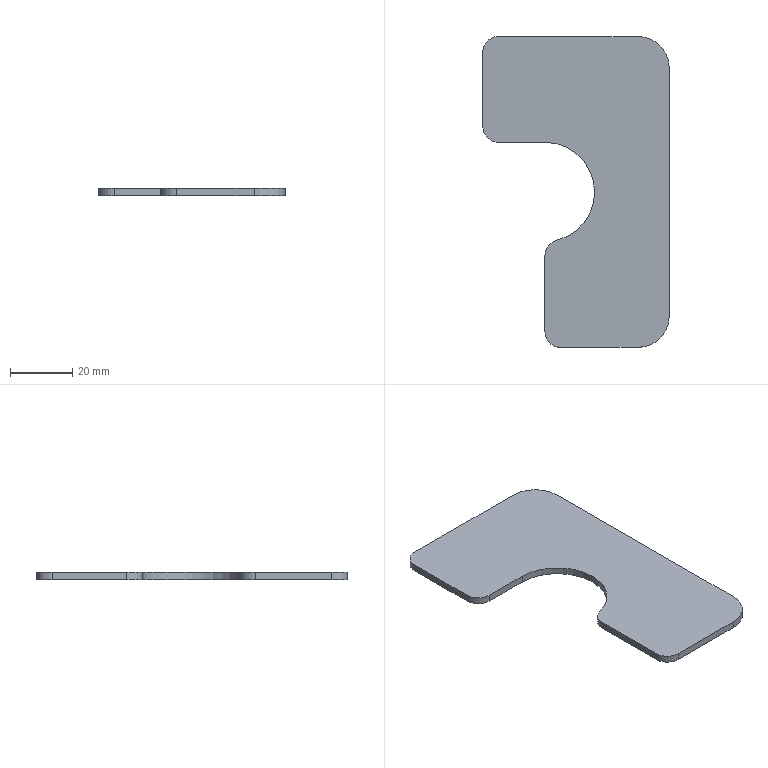Part | SolidWorks | features FlatPattern 1, SMBaseFlange 1, SheetMetal 1 | 1 solid | 15 faces | box 60 x 100 x 2.3 mm | volume 9695 mm3 | plane 8 | cylinder 7 | commonest cylinder face diameters 10 x4 20 x2 32 x1
STEP:
#1=CARTESIAN_POINT('',(247.5,0.,0.));
#2=VERTEX_POINT('',#1);
#3=CARTESIAN_POINT('',(252.5,-5.,0.));
#4=VERTEX_POINT('',#3);
#5=CARTESIAN_POINT('',(252.5,0.,0.));
#6=DIRECTION('',(0.,0.,1.));
#7=DIRECTION('',(1.,0.,0.));
#8=AXIS2_PLACEMENT_3D('',#5,#6,#7);
#9=CIRCLE('',#8,5.);
#10=EDGE_CURVE('',#2,#4,#9,.T.);
#11=ORIENTED_EDGE('',*,*,#10,.T.);
#12=CARTESIAN_POINT('',(252.5,-5.,2.3));
#13=VERTEX_POINT('',#12);
#14=CARTESIAN_POINT('',(252.5,-5.,2.3));
#15=DIRECTION('',(0.,0.,-1.));
#16=VECTOR('',#15,1000.);
#17=LINE('',#14,#16);
#18=EDGE_CURVE('',#13,#4,#17,.T.);
#19=ORIENTED_EDGE('',*,*,#18,.F.);
#20=CARTESIAN_POINT('',(247.5,0.,2.3));
#21=VERTEX_POINT('',#20);
#22=CARTESIAN_POINT('',(252.5,0.,2.3));
#23=DIRECTION('',(0.,0.,1.));
#24=DIRECTION('',(1.,0.,0.));
#25=AXIS2_PLACEMENT_3D('',#22,#23,#24);
#26=CIRCLE('',#25,5.);
#27=EDGE_CURVE('',#21,#13,#26,.T.);
#28=ORIENTED_EDGE('',*,*,#27,.F.);
#29=CARTESIAN_POINT('',(247.5,0.,2.3));
#30=DIRECTION('',(0.,0.,-1.));
#31=VECTOR('',#30,1000.);
#32=LINE('',#29,#31);
#33=EDGE_CURVE('',#21,#2,#32,.T.);
#34=ORIENTED_EDGE('',*,*,#33,.T.);
#35=EDGE_LOOP('',(#11,#19,#28,#34));
#36=FACE_OUTER_BOUND('',#35,.T.);
#37=CARTESIAN_POINT('',(252.5,0.,2.3));
#38=DIRECTION('',(0.,0.,-1.));
#39=DIRECTION('',(-1.,0.,0.));
#40=AXIS2_PLACEMENT_3D('',#37,#38,#39);
#41=CYLINDRICAL_SURFACE('',#40,5.);
#42=ADVANCED_FACE('',(#36),#41,.T.);
#43=CARTESIAN_POINT('',(277.5,-5.,0.));
#44=VERTEX_POINT('',#43);
#45=CARTESIAN_POINT('',(252.5,-5.,0.));
#46=DIRECTION('',(1.,0.,0.));
#47=VECTOR('',#46,1000.);
#48=LINE('',#45,#47);
#49=EDGE_CURVE('',#4,#44,#48,.T.);
#50=ORIENTED_EDGE('',*,*,#49,.T.);
#51=CARTESIAN_POINT('',(277.5,-5.,2.3));
#52=VERTEX_POINT('',#51);
#53=CARTESIAN_POINT('',(277.5,-5.,2.3));
#54=DIRECTION('',(0.,0.,-1.));
#55=VECTOR('',#54,1000.);
#56=LINE('',#53,#55);
#57=EDGE_CURVE('',#52,#44,#56,.T.);
#58=ORIENTED_EDGE('',*,*,#57,.F.);
#59=CARTESIAN_POINT('',(252.5,-5.,2.3));
#60=DIRECTION('',(1.,0.,0.));
#61=VECTOR('',#60,1000.);
#62=LINE('',#59,#61);
#63=EDGE_CURVE('',#13,#52,#62,.T.);
#64=ORIENTED_EDGE('',*,*,#63,.F.);
#65=ORIENTED_EDGE('',*,*,#18,.T.);
#66=EDGE_LOOP('',(#50,#58,#64,#65));
#67=FACE_OUTER_BOUND('',#66,.T.);
#68=CARTESIAN_POINT('',(252.5,-5.,2.3));
#69=DIRECTION('',(0.,1.,0.));
#70=DIRECTION('',(0.,0.,1.));
#71=AXIS2_PLACEMENT_3D('',#68,#69,#70);
#72=PLANE('',#71);
#73=ADVANCED_FACE('',(#67),#72,.F.);
#74=CARTESIAN_POINT('',(287.5,5.,0.));
#75=VERTEX_POINT('',#74);
#76=CARTESIAN_POINT('',(277.5,5.,0.));
#77=DIRECTION('',(0.,0.,1.));
#78=DIRECTION('',(-1.,0.,0.));
#79=AXIS2_PLACEMENT_3D('',#76,#77,#78);
#80=CIRCLE('',#79,10.);
#81=EDGE_CURVE('',#44,#75,#80,.T.);
#82=ORIENTED_EDGE('',*,*,#81,.T.);
#83=CARTESIAN_POINT('',(287.5,5.,2.3));
#84=VERTEX_POINT('',#83);
#85=CARTESIAN_POINT('',(287.5,5.,2.3));
#86=DIRECTION('',(0.,0.,-1.));
#87=VECTOR('',#86,1000.);
#88=LINE('',#85,#87);
#89=EDGE_CURVE('',#84,#75,#88,.T.);
#90=ORIENTED_EDGE('',*,*,#89,.F.);
#91=CARTESIAN_POINT('',(277.5,5.,2.3));
#92=DIRECTION('',(0.,0.,1.));
#93=DIRECTION('',(-1.,0.,0.));
#94=AXIS2_PLACEMENT_3D('',#91,#92,#93);
#95=CIRCLE('',#94,10.);
#96=EDGE_CURVE('',#52,#84,#95,.T.);
#97=ORIENTED_EDGE('',*,*,#96,.F.);
#98=ORIENTED_EDGE('',*,*,#57,.T.);
#99=EDGE_LOOP('',(#82,#90,#97,#98));
#100=FACE_OUTER_BOUND('',#99,.T.);
#101=CARTESIAN_POINT('',(277.5,5.,2.3));
#102=DIRECTION('',(0.,0.,-1.));
#103=DIRECTION('',(-1.,0.,0.));
#104=AXIS2_PLACEMENT_3D('',#101,#102,#103);
#105=CYLINDRICAL_SURFACE('',#104,10.);
#106=ADVANCED_FACE('',(#100),#105,.T.);
#107=CARTESIAN_POINT('',(287.5,85.,0.));
#108=VERTEX_POINT('',#107);
#109=CARTESIAN_POINT('',(287.5,85.,0.));
#110=DIRECTION('',(0.,1.,0.));
#111=VECTOR('',#110,1000.);
#112=LINE('',#109,#111);
#113=EDGE_CURVE('',#75,#108,#112,.T.);
#114=ORIENTED_EDGE('',*,*,#113,.T.);
#115=CARTESIAN_POINT('',(287.5,85.,2.3));
#116=VERTEX_POINT('',#115);
#117=CARTESIAN_POINT('',(287.5,85.,2.3));
#118=DIRECTION('',(0.,0.,-1.));
#119=VECTOR('',#118,1000.);
#120=LINE('',#117,#119);
#121=EDGE_CURVE('',#116,#108,#120,.T.);
#122=ORIENTED_EDGE('',*,*,#121,.F.);
#123=CARTESIAN_POINT('',(287.5,85.,2.3));
#124=DIRECTION('',(0.,1.,0.));
#125=VECTOR('',#124,1000.);
#126=LINE('',#123,#125);
#127=EDGE_CURVE('',#84,#116,#126,.T.);
#128=ORIENTED_EDGE('',*,*,#127,.F.);
#129=ORIENTED_EDGE('',*,*,#89,.T.);
#130=EDGE_LOOP('',(#114,#122,#128,#129));
#131=FACE_OUTER_BOUND('',#130,.T.);
#132=CARTESIAN_POINT('',(287.5,85.,2.3));
#133=DIRECTION('',(-1.,0.,0.));
#134=DIRECTION('',(0.,0.,1.));
#135=AXIS2_PLACEMENT_3D('',#132,#133,#134);
#136=PLANE('',#135);
#137=ADVANCED_FACE('',(#131),#136,.F.);
#138=CARTESIAN_POINT('',(277.5,95.,0.));
#139=VERTEX_POINT('',#138);
#140=CARTESIAN_POINT('',(277.5,85.,0.));
#141=DIRECTION('',(0.,0.,1.));
#142=DIRECTION('',(-1.,0.,0.));
#143=AXIS2_PLACEMENT_3D('',#140,#141,#142);
#144=CIRCLE('',#143,10.);
#145=EDGE_CURVE('',#108,#139,#144,.T.);
#146=ORIENTED_EDGE('',*,*,#145,.T.);
#147=CARTESIAN_POINT('',(277.5,95.,2.3));
#148=VERTEX_POINT('',#147);
#149=CARTESIAN_POINT('',(277.5,95.,2.3));
#150=DIRECTION('',(0.,0.,-1.));
#151=VECTOR('',#150,1000.);
#152=LINE('',#149,#151);
#153=EDGE_CURVE('',#148,#139,#152,.T.);
#154=ORIENTED_EDGE('',*,*,#153,.F.);
#155=CARTESIAN_POINT('',(277.5,85.,2.3));
#156=DIRECTION('',(0.,0.,1.));
#157=DIRECTION('',(-1.,0.,0.));
#158=AXIS2_PLACEMENT_3D('',#155,#156,#157);
#159=CIRCLE('',#158,10.);
#160=EDGE_CURVE('',#116,#148,#159,.T.);
#161=ORIENTED_EDGE('',*,*,#160,.F.);
#162=ORIENTED_EDGE('',*,*,#121,.T.);
#163=EDGE_LOOP('',(#146,#154,#161,#162));
#164=FACE_OUTER_BOUND('',#163,.T.);
#165=CARTESIAN_POINT('',(277.5,85.,2.3));
#166=DIRECTION('',(0.,0.,-1.));
#167=DIRECTION('',(-1.,0.,0.));
#168=AXIS2_PLACEMENT_3D('',#165,#166,#167);
#169=CYLINDRICAL_SURFACE('',#168,10.);
#170=ADVANCED_FACE('',(#164),#169,.T.);
#171=CARTESIAN_POINT('',(232.5,95.,0.));
#172=VERTEX_POINT('',#171);
#173=CARTESIAN_POINT('',(277.5,95.,0.));
#174=DIRECTION('',(-1.,0.,0.));
#175=VECTOR('',#174,1000.);
#176=LINE('',#173,#175);
#177=EDGE_CURVE('',#139,#172,#176,.T.);
#178=ORIENTED_EDGE('',*,*,#177,.T.);
#179=CARTESIAN_POINT('',(232.5,95.,2.3));
#180=VERTEX_POINT('',#179);
#181=CARTESIAN_POINT('',(232.5,95.,2.3));
#182=DIRECTION('',(0.,0.,-1.));
#183=VECTOR('',#182,1000.);
#184=LINE('',#181,#183);
#185=EDGE_CURVE('',#180,#172,#184,.T.);
#186=ORIENTED_EDGE('',*,*,#185,.F.);
#187=CARTESIAN_POINT('',(277.5,95.,2.3));
#188=DIRECTION('',(-1.,0.,0.));
#189=VECTOR('',#188,1000.);
#190=LINE('',#187,#189);
#191=EDGE_CURVE('',#148,#180,#190,.T.);
#192=ORIENTED_EDGE('',*,*,#191,.F.);
#193=ORIENTED_EDGE('',*,*,#153,.T.);
#194=EDGE_LOOP('',(#178,#186,#192,#193));
#195=FACE_OUTER_BOUND('',#194,.T.);
#196=CARTESIAN_POINT('',(277.5,95.,2.3));
#197=DIRECTION('',(0.,-1.,0.));
#198=DIRECTION('',(0.,0.,-1.));
#199=AXIS2_PLACEMENT_3D('',#196,#197,#198);
#200=PLANE('',#199);
#201=ADVANCED_FACE('',(#195),#200,.F.);
#202=CARTESIAN_POINT('',(227.5,90.,0.));
#203=VERTEX_POINT('',#202);
#204=CARTESIAN_POINT('',(232.5,90.,0.));
#205=DIRECTION('',(0.,0.,1.));
#206=DIRECTION('',(1.,0.,0.));
#207=AXIS2_PLACEMENT_3D('',#204,#205,#206);
#208=CIRCLE('',#207,5.);
#209=EDGE_CURVE('',#172,#203,#208,.T.);
#210=ORIENTED_EDGE('',*,*,#209,.T.);
#211=CARTESIAN_POINT('',(227.5,90.,2.3));
#212=VERTEX_POINT('',#211);
#213=CARTESIAN_POINT('',(227.5,90.,2.3));
#214=DIRECTION('',(0.,0.,-1.));
#215=VECTOR('',#214,1000.);
#216=LINE('',#213,#215);
#217=EDGE_CURVE('',#212,#203,#216,.T.);
#218=ORIENTED_EDGE('',*,*,#217,.F.);
#219=CARTESIAN_POINT('',(232.5,90.,2.3));
#220=DIRECTION('',(0.,0.,1.));
#221=DIRECTION('',(1.,0.,0.));
#222=AXIS2_PLACEMENT_3D('',#219,#220,#221);
#223=CIRCLE('',#222,5.);
#224=EDGE_CURVE('',#180,#212,#223,.T.);
#225=ORIENTED_EDGE('',*,*,#224,.F.);
#226=ORIENTED_EDGE('',*,*,#185,.T.);
#227=EDGE_LOOP('',(#210,#218,#225,#226));
#228=FACE_OUTER_BOUND('',#227,.T.);
#229=CARTESIAN_POINT('',(232.5,90.,2.3));
#230=DIRECTION('',(0.,0.,-1.));
#231=DIRECTION('',(-1.,0.,0.));
#232=AXIS2_PLACEMENT_3D('',#229,#230,#231);
#233=CYLINDRICAL_SURFACE('',#232,5.);
#234=ADVANCED_FACE('',(#228),#233,.T.);
#235=CARTESIAN_POINT('',(227.5,66.,0.));
#236=VERTEX_POINT('',#235);
#237=CARTESIAN_POINT('',(227.5,90.,0.));
#238=DIRECTION('',(0.,-1.,0.));
#239=VECTOR('',#238,1000.);
#240=LINE('',#237,#239);
#241=EDGE_CURVE('',#203,#236,#240,.T.);
#242=ORIENTED_EDGE('',*,*,#241,.T.);
#243=CARTESIAN_POINT('',(227.5,66.,2.3));
#244=VERTEX_POINT('',#243);
#245=CARTESIAN_POINT('',(227.5,66.,2.3));
#246=DIRECTION('',(0.,0.,-1.));
#247=VECTOR('',#246,1000.);
#248=LINE('',#245,#247);
#249=EDGE_CURVE('',#244,#236,#248,.T.);
#250=ORIENTED_EDGE('',*,*,#249,.F.);
#251=CARTESIAN_POINT('',(227.5,90.,2.3));
#252=DIRECTION('',(0.,-1.,0.));
#253=VECTOR('',#252,1000.);
#254=LINE('',#251,#253);
#255=EDGE_CURVE('',#212,#244,#254,.T.);
#256=ORIENTED_EDGE('',*,*,#255,.F.);
#257=ORIENTED_EDGE('',*,*,#217,.T.);
#258=EDGE_LOOP('',(#242,#250,#256,#257));
#259=FACE_OUTER_BOUND('',#258,.T.);
#260=CARTESIAN_POINT('',(227.5,90.,2.3));
#261=DIRECTION('',(1.,0.,0.));
#262=DIRECTION('',(0.,0.,-1.));
#263=AXIS2_PLACEMENT_3D('',#260,#261,#262);
#264=PLANE('',#263);
#265=ADVANCED_FACE('',(#259),#264,.F.);
#266=CARTESIAN_POINT('',(232.5,61.,0.));
#267=VERTEX_POINT('',#266);
#268=CARTESIAN_POINT('',(232.5,66.,0.));
#269=DIRECTION('',(0.,0.,1.));
#270=DIRECTION('',(1.,0.,0.));
#271=AXIS2_PLACEMENT_3D('',#268,#269,#270);
#272=CIRCLE('',#271,5.);
#273=EDGE_CURVE('',#236,#267,#272,.T.);
#274=ORIENTED_EDGE('',*,*,#273,.T.);
#275=CARTESIAN_POINT('',(232.5,61.,2.3));
#276=VERTEX_POINT('',#275);
#277=CARTESIAN_POINT('',(232.5,61.,2.3));
#278=DIRECTION('',(0.,0.,-1.));
#279=VECTOR('',#278,1000.);
#280=LINE('',#277,#279);
#281=EDGE_CURVE('',#276,#267,#280,.T.);
#282=ORIENTED_EDGE('',*,*,#281,.F.);
#283=CARTESIAN_POINT('',(232.5,66.,2.3));
#284=DIRECTION('',(0.,0.,1.));
#285=DIRECTION('',(1.,0.,0.));
#286=AXIS2_PLACEMENT_3D('',#283,#284,#285);
#287=CIRCLE('',#286,5.);
#288=EDGE_CURVE('',#244,#276,#287,.T.);
#289=ORIENTED_EDGE('',*,*,#288,.F.);
#290=ORIENTED_EDGE('',*,*,#249,.T.);
#291=EDGE_LOOP('',(#274,#282,#289,#290));
#292=FACE_OUTER_BOUND('',#291,.T.);
#293=CARTESIAN_POINT('',(232.5,66.,2.3));
#294=DIRECTION('',(0.,0.,-1.));
#295=DIRECTION('',(-1.,0.,0.));
#296=AXIS2_PLACEMENT_3D('',#293,#294,#295);
#297=CYLINDRICAL_SURFACE('',#296,5.);
#298=ADVANCED_FACE('',(#292),#297,.T.);
#299=CARTESIAN_POINT('',(247.5,61.,0.));
#300=VERTEX_POINT('',#299);
#301=CARTESIAN_POINT('',(232.5,61.,0.));
#302=DIRECTION('',(1.,0.,0.));
#303=VECTOR('',#302,1000.);
#304=LINE('',#301,#303);
#305=EDGE_CURVE('',#267,#300,#304,.T.);
#306=ORIENTED_EDGE('',*,*,#305,.T.);
#307=CARTESIAN_POINT('',(247.5,61.,2.3));
#308=VERTEX_POINT('',#307);
#309=CARTESIAN_POINT('',(247.5,61.,2.3));
#310=DIRECTION('',(0.,0.,-1.));
#311=VECTOR('',#310,1000.);
#312=LINE('',#309,#311);
#313=EDGE_CURVE('',#308,#300,#312,.T.);
#314=ORIENTED_EDGE('',*,*,#313,.F.);
#315=CARTESIAN_POINT('',(232.5,61.,2.3));
#316=DIRECTION('',(1.,0.,0.));
#317=VECTOR('',#316,1000.);
#318=LINE('',#315,#317);
#319=EDGE_CURVE('',#276,#308,#318,.T.);
#320=ORIENTED_EDGE('',*,*,#319,.F.);
#321=ORIENTED_EDGE('',*,*,#281,.T.);
#322=EDGE_LOOP('',(#306,#314,#320,#321));
#323=FACE_OUTER_BOUND('',#322,.T.);
#324=CARTESIAN_POINT('',(232.5,61.,2.3));
#325=DIRECTION('',(0.,1.,0.));
#326=DIRECTION('',(0.,0.,1.));
#327=AXIS2_PLACEMENT_3D('',#324,#325,#326);
#328=PLANE('',#327);
#329=ADVANCED_FACE('',(#323),#328,.F.);
#330=CARTESIAN_POINT('',(251.31,29.46,0.));
#331=VERTEX_POINT('',#330);
#332=CARTESIAN_POINT('',(247.5,45.,0.));
#333=DIRECTION('',(0.,0.,-1.));
#334=DIRECTION('',(1.,0.,0.));
#335=AXIS2_PLACEMENT_3D('',#332,#333,#334);
#336=CIRCLE('',#335,16.);
#337=EDGE_CURVE('',#300,#331,#336,.T.);
#338=ORIENTED_EDGE('',*,*,#337,.T.);
#339=CARTESIAN_POINT('',(251.31,29.46,2.3));
#340=VERTEX_POINT('',#339);
#341=CARTESIAN_POINT('',(251.31,29.46,2.3));
#342=DIRECTION('',(0.,0.,-1.));
#343=VECTOR('',#342,1000.);
#344=LINE('',#341,#343);
#345=EDGE_CURVE('',#340,#331,#344,.T.);
#346=ORIENTED_EDGE('',*,*,#345,.F.);
#347=CARTESIAN_POINT('',(247.5,45.,2.3));
#348=DIRECTION('',(0.,0.,-1.));
#349=DIRECTION('',(1.,0.,0.));
#350=AXIS2_PLACEMENT_3D('',#347,#348,#349);
#351=CIRCLE('',#350,16.);
#352=EDGE_CURVE('',#308,#340,#351,.T.);
#353=ORIENTED_EDGE('',*,*,#352,.F.);
#354=ORIENTED_EDGE('',*,*,#313,.T.);
#355=EDGE_LOOP('',(#338,#346,#353,#354));
#356=FACE_OUTER_BOUND('',#355,.T.);
#357=CARTESIAN_POINT('',(247.5,45.,2.3));
#358=DIRECTION('',(0.,0.,-1.));
#359=DIRECTION('',(-1.,0.,0.));
#360=AXIS2_PLACEMENT_3D('',#357,#358,#359);
#361=CYLINDRICAL_SURFACE('',#360,16.);
#362=ADVANCED_FACE('',(#356),#361,.F.);
#363=CARTESIAN_POINT('',(247.5,24.604,0.));
#364=VERTEX_POINT('',#363);
#365=CARTESIAN_POINT('',(252.5,24.604,0.));
#366=DIRECTION('',(0.,0.,1.));
#367=DIRECTION('',(-1.,0.,0.));
#368=AXIS2_PLACEMENT_3D('',#365,#366,#367);
#369=CIRCLE('',#368,5.);
#370=EDGE_CURVE('',#331,#364,#369,.T.);
#371=ORIENTED_EDGE('',*,*,#370,.T.);
#372=CARTESIAN_POINT('',(247.5,24.604,2.3));
#373=VERTEX_POINT('',#372);
#374=CARTESIAN_POINT('',(247.5,24.604,2.3));
#375=DIRECTION('',(0.,0.,-1.));
#376=VECTOR('',#375,1000.);
#377=LINE('',#374,#376);
#378=EDGE_CURVE('',#373,#364,#377,.T.);
#379=ORIENTED_EDGE('',*,*,#378,.F.);
#380=CARTESIAN_POINT('',(252.5,24.604,2.3));
#381=DIRECTION('',(0.,0.,1.));
#382=DIRECTION('',(-1.,0.,0.));
#383=AXIS2_PLACEMENT_3D('',#380,#381,#382);
#384=CIRCLE('',#383,5.);
#385=EDGE_CURVE('',#340,#373,#384,.T.);
#386=ORIENTED_EDGE('',*,*,#385,.F.);
#387=ORIENTED_EDGE('',*,*,#345,.T.);
#388=EDGE_LOOP('',(#371,#379,#386,#387));
#389=FACE_OUTER_BOUND('',#388,.T.);
#390=CARTESIAN_POINT('',(252.5,24.604,2.3));
#391=DIRECTION('',(0.,0.,-1.));
#392=DIRECTION('',(-1.,0.,0.));
#393=AXIS2_PLACEMENT_3D('',#390,#391,#392);
#394=CYLINDRICAL_SURFACE('',#393,5.);
#395=ADVANCED_FACE('',(#389),#394,.T.);
#396=CARTESIAN_POINT('',(247.5,24.604,0.));
#397=DIRECTION('',(0.,-1.,0.));
#398=VECTOR('',#397,1000.);
#399=LINE('',#396,#398);
#400=EDGE_CURVE('',#364,#2,#399,.T.);
#401=ORIENTED_EDGE('',*,*,#400,.T.);
#402=ORIENTED_EDGE('',*,*,#33,.F.);
#403=CARTESIAN_POINT('',(247.5,24.604,2.3));
#404=DIRECTION('',(0.,-1.,0.));
#405=VECTOR('',#404,1000.);
#406=LINE('',#403,#405);
#407=EDGE_CURVE('',#373,#21,#406,.T.);
#408=ORIENTED_EDGE('',*,*,#407,.F.);
#409=ORIENTED_EDGE('',*,*,#378,.T.);
#410=EDGE_LOOP('',(#401,#402,#408,#409));
#411=FACE_OUTER_BOUND('',#410,.T.);
#412=CARTESIAN_POINT('',(247.5,24.604,2.3));
#413=DIRECTION('',(1.,0.,0.));
#414=DIRECTION('',(0.,0.,-1.));
#415=AXIS2_PLACEMENT_3D('',#412,#413,#414);
#416=PLANE('',#415);
#417=ADVANCED_FACE('',(#411),#416,.F.);
#418=ORIENTED_EDGE('',*,*,#27,.T.);
#419=ORIENTED_EDGE('',*,*,#63,.T.);
#420=ORIENTED_EDGE('',*,*,#96,.T.);
#421=ORIENTED_EDGE('',*,*,#127,.T.);
#422=ORIENTED_EDGE('',*,*,#160,.T.);
#423=ORIENTED_EDGE('',*,*,#191,.T.);
#424=ORIENTED_EDGE('',*,*,#224,.T.);
#425=ORIENTED_EDGE('',*,*,#255,.T.);
#426=ORIENTED_EDGE('',*,*,#288,.T.);
#427=ORIENTED_EDGE('',*,*,#319,.T.);
#428=ORIENTED_EDGE('',*,*,#352,.T.);
#429=ORIENTED_EDGE('',*,*,#385,.T.);
#430=ORIENTED_EDGE('',*,*,#407,.T.);
#431=EDGE_LOOP('',(#418,#419,#420,#421,#422,#423,#424,#425,#426,#427,#428,#429,#430));
#432=FACE_OUTER_BOUND('',#431,.T.);
#433=CARTESIAN_POINT('',(252.5,0.,2.3));
#434=DIRECTION('',(0.,0.,1.));
#435=DIRECTION('',(1.,0.,0.));
#436=AXIS2_PLACEMENT_3D('',#433,#434,#435);
#437=PLANE('',#436);
#438=ADVANCED_FACE('',(#432),#437,.T.);
#439=ORIENTED_EDGE('',*,*,#10,.F.);
#440=ORIENTED_EDGE('',*,*,#400,.F.);
#441=ORIENTED_EDGE('',*,*,#370,.F.);
#442=ORIENTED_EDGE('',*,*,#337,.F.);
#443=ORIENTED_EDGE('',*,*,#305,.F.);
#444=ORIENTED_EDGE('',*,*,#273,.F.);
#445=ORIENTED_EDGE('',*,*,#241,.F.);
#446=ORIENTED_EDGE('',*,*,#209,.F.);
#447=ORIENTED_EDGE('',*,*,#177,.F.);
#448=ORIENTED_EDGE('',*,*,#145,.F.);
#449=ORIENTED_EDGE('',*,*,#113,.F.);
#450=ORIENTED_EDGE('',*,*,#81,.F.);
#451=ORIENTED_EDGE('',*,*,#49,.F.);
#452=EDGE_LOOP('',(#439,#440,#441,#442,#443,#444,#445,#446,#447,#448,#449,#450,#451));
#453=FACE_OUTER_BOUND('',#452,.T.);
#454=CARTESIAN_POINT('',(252.5,0.,0.));
#455=DIRECTION('',(0.,0.,1.));
#456=DIRECTION('',(1.,0.,0.));
#457=AXIS2_PLACEMENT_3D('',#454,#455,#456);
#458=PLANE('',#457);
#459=ADVANCED_FACE('',(#453),#458,.F.);
#460=CLOSED_SHELL('',(#42,#73,#106,#137,#170,#201,#234,#265,#298,#329,#362,#395,#417,#438,#459));
#461=MANIFOLD_SOLID_BREP('',#460);
#462=CARTESIAN_POINT('',(0.,0.,0.));
#463=DIRECTION('',(0.,0.,1.));
#464=DIRECTION('',(1.,0.,0.));
#465=AXIS2_PLACEMENT_3D('',#462,#463,#464);
#466=(LENGTH_UNIT()NAMED_UNIT(*)SI_UNIT(.MILLI.,.METRE.));
#467=UNCERTAINTY_MEASURE_WITH_UNIT(LENGTH_MEASURE(0.00001),#466,'','');
#468=(NAMED_UNIT(*)PLANE_ANGLE_UNIT()SI_UNIT($,.RADIAN.));
#469=(NAMED_UNIT(*)SI_UNIT($,.STERADIAN.)SOLID_ANGLE_UNIT());
#470=(GEOMETRIC_REPRESENTATION_CONTEXT(3)GLOBAL_UNCERTAINTY_ASSIGNED_CONTEXT((#467))GLOBAL_UNIT_ASSIGNED_CONTEXT((#466,#468,#469))REPRESENTATION_CONTEXT('',''));
#471=ADVANCED_BREP_SHAPE_REPRESENTATION('',(#461,#465),#470);